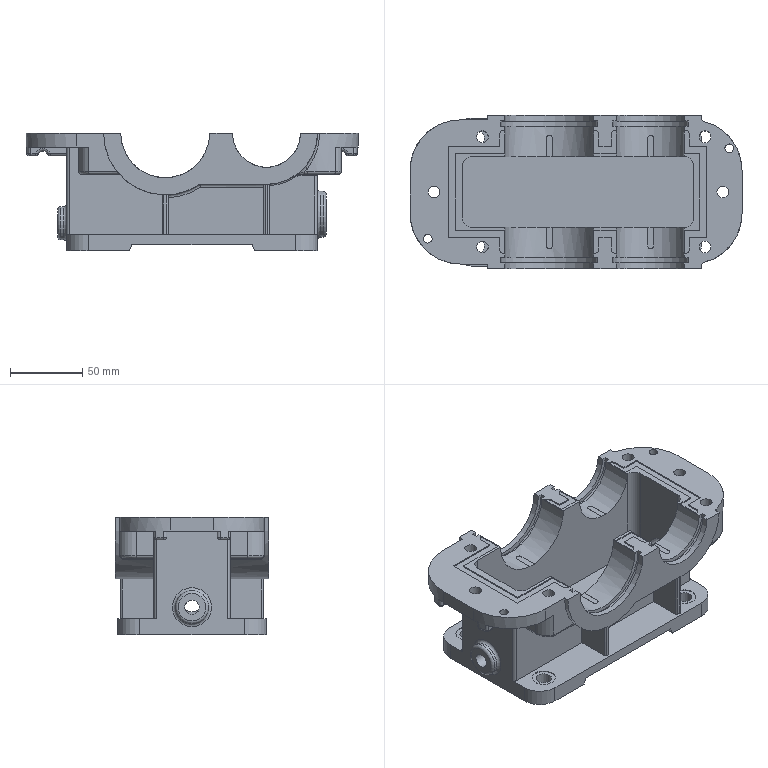Part | NX | features EXTRUDE 28, BLEND 23, DATUM_CSYS 21, SKETCH 20, EXTRACT_STRING 8, Instance Feature 4, MIRROR_CURVE 4, Mirror Feature 4, DATUM_PLANE 3, FACE_BLEND 3, RIB 3, CPROJ 2, REPLACE_FACE 2, U_SLOT 2, SYMBOLIC_THREAD 1 | 1 solid | 344 faces | box 229.56 x 106.4 x 81.2 mm | volume 501453 mm3 | plane 144 | cylinder 134 | torus 36 | sphere 24 | spline 6 | commonest cylinder face diameters 4 x58 2 x10 6.8 x8 8.2 x6 6.863 x4 10.5 x4